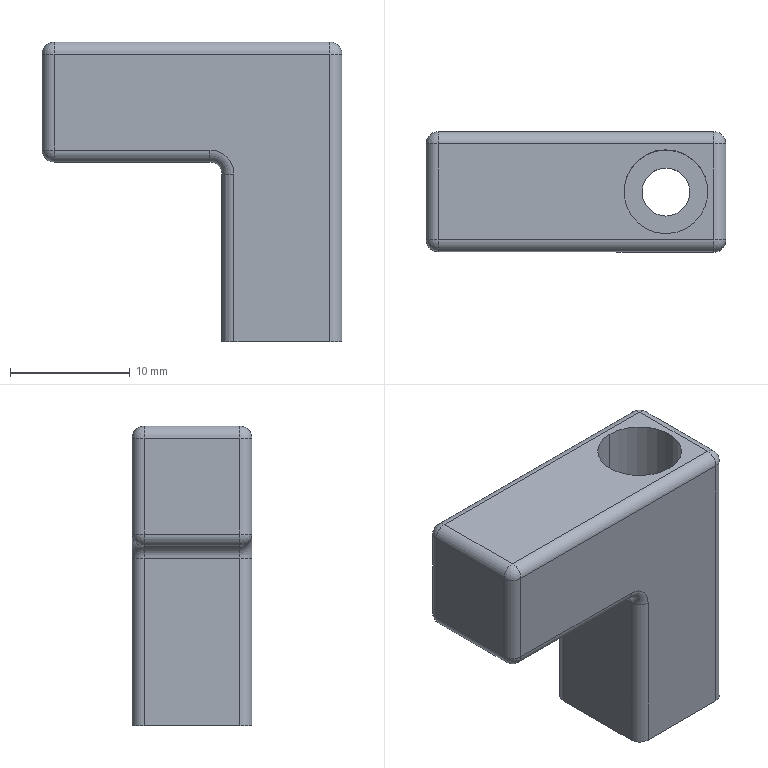Part | NX | 1 solid | 35 faces | box 25 x 10 x 25 mm | volume 3255 mm3 | cylinder 18 | plane 9 | sphere 6 | torus 2 | commonest cylinder face diameters 2 x14 4 x2 7 x2
STEP:
#1=CARTESIAN_POINT('',(12.5,-4.,-25.));
#2=VERTEX_POINT('',#1);
#3=CARTESIAN_POINT('',(12.5,4.,-25.));
#4=VERTEX_POINT('',#3);
#5=CARTESIAN_POINT('',(12.5,-4.,-25.));
#6=DIRECTION('',(0.,1.,0.));
#7=VECTOR('',#6,1000.);
#8=LINE('',#5,#7);
#9=EDGE_CURVE('',#2,#4,#8,.T.);
#10=ORIENTED_EDGE('',*,*,#9,.F.);
#11=CARTESIAN_POINT('',(11.5,-5.,-25.));
#12=VERTEX_POINT('',#11);
#13=CARTESIAN_POINT('',(11.5,-4.,-25.));
#14=DIRECTION('',(0.,0.,-1.));
#15=DIRECTION('',(1.,0.,0.));
#16=AXIS2_PLACEMENT_3D('',#13,#14,#15);
#17=CIRCLE('',#16,1.);
#18=EDGE_CURVE('',#2,#12,#17,.T.);
#19=ORIENTED_EDGE('',*,*,#18,.T.);
#20=CARTESIAN_POINT('',(3.5,-5.,-25.));
#21=VERTEX_POINT('',#20);
#22=CARTESIAN_POINT('',(3.5,-5.,-25.));
#23=DIRECTION('',(1.,0.,0.));
#24=VECTOR('',#23,1000.);
#25=LINE('',#22,#24);
#26=EDGE_CURVE('',#21,#12,#25,.T.);
#27=ORIENTED_EDGE('',*,*,#26,.F.);
#28=CARTESIAN_POINT('',(2.5,-4.,-25.));
#29=VERTEX_POINT('',#28);
#30=CARTESIAN_POINT('',(3.5,-4.,-25.));
#31=DIRECTION('',(0.,0.,-1.));
#32=DIRECTION('',(0.,-1.,0.));
#33=AXIS2_PLACEMENT_3D('',#30,#31,#32);
#34=CIRCLE('',#33,1.);
#35=EDGE_CURVE('',#21,#29,#34,.T.);
#36=ORIENTED_EDGE('',*,*,#35,.T.);
#37=CARTESIAN_POINT('',(2.5,4.,-25.));
#38=VERTEX_POINT('',#37);
#39=CARTESIAN_POINT('',(2.5,4.,-25.));
#40=DIRECTION('',(0.,-1.,0.));
#41=VECTOR('',#40,1000.);
#42=LINE('',#39,#41);
#43=EDGE_CURVE('',#38,#29,#42,.T.);
#44=ORIENTED_EDGE('',*,*,#43,.F.);
#45=CARTESIAN_POINT('',(3.5,5.,-25.));
#46=VERTEX_POINT('',#45);
#47=CARTESIAN_POINT('',(3.5,4.,-25.));
#48=DIRECTION('',(0.,0.,-1.));
#49=DIRECTION('',(-1.,0.,0.));
#50=AXIS2_PLACEMENT_3D('',#47,#48,#49);
#51=CIRCLE('',#50,1.);
#52=EDGE_CURVE('',#38,#46,#51,.T.);
#53=ORIENTED_EDGE('',*,*,#52,.T.);
#54=CARTESIAN_POINT('',(11.5,5.,-25.));
#55=VERTEX_POINT('',#54);
#56=CARTESIAN_POINT('',(11.5,5.,-25.));
#57=DIRECTION('',(-1.,0.,0.));
#58=VECTOR('',#57,1000.);
#59=LINE('',#56,#58);
#60=EDGE_CURVE('',#55,#46,#59,.T.);
#61=ORIENTED_EDGE('',*,*,#60,.F.);
#62=CARTESIAN_POINT('',(11.5,4.,-25.));
#63=DIRECTION('',(0.,0.,-1.));
#64=DIRECTION('',(0.,1.,0.));
#65=AXIS2_PLACEMENT_3D('',#62,#63,#64);
#66=CIRCLE('',#65,1.);
#67=EDGE_CURVE('',#55,#4,#66,.T.);
#68=ORIENTED_EDGE('',*,*,#67,.T.);
#69=EDGE_LOOP('',(#10,#19,#27,#36,#44,#53,#61,#68));
#70=FACE_BOUND('',#69,.T.);
#71=CARTESIAN_POINT('',(7.5,-2.,-25.));
#72=VERTEX_POINT('',#71);
#73=CARTESIAN_POINT('',(7.5,2.,-25.));
#74=VERTEX_POINT('',#73);
#75=CARTESIAN_POINT('',(7.5,0.,-25.));
#76=DIRECTION('',(0.,0.,1.));
#77=DIRECTION('',(0.,-1.,0.));
#78=AXIS2_PLACEMENT_3D('',#75,#76,#77);
#79=CIRCLE('',#78,2.);
#80=EDGE_CURVE('',#72,#74,#79,.T.);
#81=ORIENTED_EDGE('',*,*,#80,.T.);
#82=CARTESIAN_POINT('',(7.5,0.,-25.));
#83=DIRECTION('',(0.,0.,1.));
#84=DIRECTION('',(0.,1.,0.));
#85=AXIS2_PLACEMENT_3D('',#82,#83,#84);
#86=CIRCLE('',#85,2.);
#87=EDGE_CURVE('',#74,#72,#86,.T.);
#88=ORIENTED_EDGE('',*,*,#87,.T.);
#89=EDGE_LOOP('',(#81,#88));
#90=FACE_BOUND('',#89,.T.);
#91=CARTESIAN_POINT('',(2.5,-26.5,-25.));
#92=DIRECTION('',(0.,0.,1.));
#93=DIRECTION('',(0.,-1.,0.));
#94=AXIS2_PLACEMENT_3D('',#91,#92,#93);
#95=PLANE('',#94);
#96=ADVANCED_FACE('',(#70,#90),#95,.F.);
#97=CARTESIAN_POINT('',(12.5,4.,-1.));
#98=VERTEX_POINT('',#97);
#99=CARTESIAN_POINT('',(12.5,4.,-25.));
#100=DIRECTION('',(0.,0.,1.));
#101=VECTOR('',#100,1000.);
#102=LINE('',#99,#101);
#103=EDGE_CURVE('',#4,#98,#102,.T.);
#104=ORIENTED_EDGE('',*,*,#103,.F.);
#105=ORIENTED_EDGE('',*,*,#67,.F.);
#106=CARTESIAN_POINT('',(11.5,5.,-1.));
#107=VERTEX_POINT('',#106);
#108=CARTESIAN_POINT('',(11.5,5.,-25.));
#109=DIRECTION('',(0.,0.,1.));
#110=VECTOR('',#109,1000.);
#111=LINE('',#108,#110);
#112=EDGE_CURVE('',#55,#107,#111,.T.);
#113=ORIENTED_EDGE('',*,*,#112,.T.);
#114=CARTESIAN_POINT('',(11.5,4.,-1.));
#115=DIRECTION('',(0.,0.,1.));
#116=DIRECTION('',(1.,0.,0.));
#117=AXIS2_PLACEMENT_3D('',#114,#115,#116);
#118=CIRCLE('',#117,1.);
#119=EDGE_CURVE('',#98,#107,#118,.T.);
#120=ORIENTED_EDGE('',*,*,#119,.F.);
#121=EDGE_LOOP('',(#104,#105,#113,#120));
#122=FACE_BOUND('',#121,.T.);
#123=CARTESIAN_POINT('',(11.5,4.,-57.59));
#124=DIRECTION('',(0.,0.,1.));
#125=DIRECTION('',(-1.,0.,0.));
#126=AXIS2_PLACEMENT_3D('',#123,#124,#125);
#127=CYLINDRICAL_SURFACE('',#126,1.);
#128=ADVANCED_FACE('',(#122),#127,.T.);
#129=CARTESIAN_POINT('',(11.5,4.,0.));
#130=VERTEX_POINT('',#129);
#131=CARTESIAN_POINT('',(11.5,4.,-1.));
#132=DIRECTION('',(-1.,0.,0.));
#133=DIRECTION('',(0.,0.,1.));
#134=AXIS2_PLACEMENT_3D('',#131,#132,#133);
#135=CIRCLE('',#134,1.);
#136=EDGE_CURVE('',#130,#107,#135,.T.);
#137=ORIENTED_EDGE('',*,*,#136,.F.);
#138=CARTESIAN_POINT('',(11.5,4.,-1.));
#139=DIRECTION('',(0.,1.,0.));
#140=DIRECTION('',(0.,0.,1.));
#141=AXIS2_PLACEMENT_3D('',#138,#139,#140);
#142=CIRCLE('',#141,1.);
#143=EDGE_CURVE('',#130,#98,#142,.T.);
#144=ORIENTED_EDGE('',*,*,#143,.T.);
#145=ORIENTED_EDGE('',*,*,#119,.T.);
#146=EDGE_LOOP('',(#137,#144,#145));
#147=FACE_BOUND('',#146,.T.);
#148=CARTESIAN_POINT('',(11.5,4.,-1.));
#149=DIRECTION('',(0.7071,-0.7071,0.));
#150=DIRECTION('',(-0.7071,-0.7071,0.));
#151=AXIS2_PLACEMENT_3D('',#148,#149,#150);
#152=SPHERICAL_SURFACE('',#151,1.);
#153=ADVANCED_FACE('',(#147),#152,.T.);
#154=CARTESIAN_POINT('',(11.5,-4.,0.));
#155=VERTEX_POINT('',#154);
#156=CARTESIAN_POINT('',(12.5,-4.,-1.));
#157=VERTEX_POINT('',#156);
#158=CARTESIAN_POINT('',(11.5,-4.,-1.));
#159=DIRECTION('',(0.,1.,0.));
#160=DIRECTION('',(0.,0.,1.));
#161=AXIS2_PLACEMENT_3D('',#158,#159,#160);
#162=CIRCLE('',#161,1.);
#163=EDGE_CURVE('',#155,#157,#162,.T.);
#164=ORIENTED_EDGE('',*,*,#163,.T.);
#165=CARTESIAN_POINT('',(12.5,-4.,-1.));
#166=DIRECTION('',(0.,1.,0.));
#167=VECTOR('',#166,1000.);
#168=LINE('',#165,#167);
#169=EDGE_CURVE('',#157,#98,#168,.T.);
#170=ORIENTED_EDGE('',*,*,#169,.T.);
#171=ORIENTED_EDGE('',*,*,#143,.F.);
#172=CARTESIAN_POINT('',(11.5,-4.,0.));
#173=DIRECTION('',(0.,1.,0.));
#174=VECTOR('',#173,1000.);
#175=LINE('',#172,#174);
#176=EDGE_CURVE('',#155,#130,#175,.T.);
#177=ORIENTED_EDGE('',*,*,#176,.F.);
#178=EDGE_LOOP('',(#164,#170,#171,#177));
#179=FACE_BOUND('',#178,.T.);
#180=CARTESIAN_POINT('',(11.5,-4.056,-1.));
#181=DIRECTION('',(0.,1.,0.));
#182=DIRECTION('',(0.,0.,-1.));
#183=AXIS2_PLACEMENT_3D('',#180,#181,#182);
#184=CYLINDRICAL_SURFACE('',#183,1.);
#185=ADVANCED_FACE('',(#179),#184,.T.);
#186=CARTESIAN_POINT('',(-11.5,-4.,0.));
#187=VERTEX_POINT('',#186);
#188=CARTESIAN_POINT('',(-11.5,-4.,0.));
#189=DIRECTION('',(1.,0.,0.));
#190=VECTOR('',#189,1000.);
#191=LINE('',#188,#190);
#192=EDGE_CURVE('',#187,#155,#191,.T.);
#193=ORIENTED_EDGE('',*,*,#192,.T.);
#194=ORIENTED_EDGE('',*,*,#176,.T.);
#195=CARTESIAN_POINT('',(-11.5,4.,0.));
#196=VERTEX_POINT('',#195);
#197=CARTESIAN_POINT('',(11.5,4.,0.));
#198=DIRECTION('',(-1.,0.,0.));
#199=VECTOR('',#198,1000.);
#200=LINE('',#197,#199);
#201=EDGE_CURVE('',#130,#196,#200,.T.);
#202=ORIENTED_EDGE('',*,*,#201,.T.);
#203=CARTESIAN_POINT('',(-11.5,4.,0.));
#204=DIRECTION('',(0.,-1.,0.));
#205=VECTOR('',#204,1000.);
#206=LINE('',#203,#205);
#207=EDGE_CURVE('',#196,#187,#206,.T.);
#208=ORIENTED_EDGE('',*,*,#207,.T.);
#209=EDGE_LOOP('',(#193,#194,#202,#208));
#210=FACE_BOUND('',#209,.T.);
#211=CARTESIAN_POINT('',(7.5,-3.5,0.));
#212=VERTEX_POINT('',#211);
#213=CARTESIAN_POINT('',(7.5,3.5,0.));
#214=VERTEX_POINT('',#213);
#215=CARTESIAN_POINT('',(7.5,0.,0.));
#216=DIRECTION('',(0.,0.,1.));
#217=DIRECTION('',(0.,-1.,0.));
#218=AXIS2_PLACEMENT_3D('',#215,#216,#217);
#219=CIRCLE('',#218,3.5);
#220=EDGE_CURVE('',#212,#214,#219,.T.);
#221=ORIENTED_EDGE('',*,*,#220,.F.);
#222=CARTESIAN_POINT('',(7.5,0.,0.));
#223=DIRECTION('',(0.,0.,1.));
#224=DIRECTION('',(0.,1.,0.));
#225=AXIS2_PLACEMENT_3D('',#222,#223,#224);
#226=CIRCLE('',#225,3.5);
#227=EDGE_CURVE('',#214,#212,#226,.T.);
#228=ORIENTED_EDGE('',*,*,#227,.F.);
#229=EDGE_LOOP('',(#221,#228));
#230=FACE_BOUND('',#229,.T.);
#231=CARTESIAN_POINT('',(4.5,-26.5,0.));
#232=DIRECTION('',(0.,0.,1.));
#233=DIRECTION('',(0.,-1.,0.));
#234=AXIS2_PLACEMENT_3D('',#231,#232,#233);
#235=PLANE('',#234);
#236=ADVANCED_FACE('',(#210,#230),#235,.T.);
#237=CARTESIAN_POINT('',(7.5,-3.5,-15.));
#238=VERTEX_POINT('',#237);
#239=CARTESIAN_POINT('',(7.5,-3.5,0.));
#240=DIRECTION('',(0.,0.,-1.));
#241=VECTOR('',#240,1000.);
#242=LINE('',#239,#241);
#243=EDGE_CURVE('',#212,#238,#242,.T.);
#244=ORIENTED_EDGE('',*,*,#243,.T.);
#245=CARTESIAN_POINT('',(7.5,3.5,-15.));
#246=VERTEX_POINT('',#245);
#247=CARTESIAN_POINT('',(7.5,0.,-15.));
#248=DIRECTION('',(0.,0.,1.));
#249=DIRECTION('',(0.,1.,0.));
#250=AXIS2_PLACEMENT_3D('',#247,#248,#249);
#251=CIRCLE('',#250,3.5);
#252=EDGE_CURVE('',#246,#238,#251,.T.);
#253=ORIENTED_EDGE('',*,*,#252,.F.);
#254=CARTESIAN_POINT('',(7.5,3.5,0.));
#255=DIRECTION('',(0.,0.,-1.));
#256=VECTOR('',#255,1000.);
#257=LINE('',#254,#256);
#258=EDGE_CURVE('',#214,#246,#257,.T.);
#259=ORIENTED_EDGE('',*,*,#258,.F.);
#260=ORIENTED_EDGE('',*,*,#227,.T.);
#261=EDGE_LOOP('',(#244,#253,#259,#260));
#262=FACE_BOUND('',#261,.T.);
#263=CARTESIAN_POINT('',(7.5,0.,0.));
#264=DIRECTION('',(0.,0.,1.));
#265=DIRECTION('',(0.,-1.,0.));
#266=AXIS2_PLACEMENT_3D('',#263,#264,#265);
#267=CYLINDRICAL_SURFACE('',#266,3.5);
#268=ADVANCED_FACE('',(#262),#267,.F.);
#269=ORIENTED_EDGE('',*,*,#258,.T.);
#270=CARTESIAN_POINT('',(7.5,0.,-15.));
#271=DIRECTION('',(0.,0.,1.));
#272=DIRECTION('',(0.,-1.,0.));
#273=AXIS2_PLACEMENT_3D('',#270,#271,#272);
#274=CIRCLE('',#273,3.5);
#275=EDGE_CURVE('',#238,#246,#274,.T.);
#276=ORIENTED_EDGE('',*,*,#275,.F.);
#277=ORIENTED_EDGE('',*,*,#243,.F.);
#278=ORIENTED_EDGE('',*,*,#220,.T.);
#279=EDGE_LOOP('',(#269,#276,#277,#278));
#280=FACE_BOUND('',#279,.T.);
#281=CARTESIAN_POINT('',(7.5,0.,0.));
#282=DIRECTION('',(0.,0.,1.));
#283=DIRECTION('',(0.,-1.,0.));
#284=AXIS2_PLACEMENT_3D('',#281,#282,#283);
#285=CYLINDRICAL_SURFACE('',#284,3.5);
#286=ADVANCED_FACE('',(#280),#285,.F.);
#287=ORIENTED_EDGE('',*,*,#275,.T.);
#288=ORIENTED_EDGE('',*,*,#252,.T.);
#289=EDGE_LOOP('',(#287,#288));
#290=FACE_BOUND('',#289,.T.);
#291=CARTESIAN_POINT('',(7.5,-2.,-15.));
#292=VERTEX_POINT('',#291);
#293=CARTESIAN_POINT('',(7.5,2.,-15.));
#294=VERTEX_POINT('',#293);
#295=CARTESIAN_POINT('',(7.5,0.,-15.));
#296=DIRECTION('',(0.,0.,1.));
#297=DIRECTION('',(0.,-1.,0.));
#298=AXIS2_PLACEMENT_3D('',#295,#296,#297);
#299=CIRCLE('',#298,2.);
#300=EDGE_CURVE('',#292,#294,#299,.T.);
#301=ORIENTED_EDGE('',*,*,#300,.F.);
#302=CARTESIAN_POINT('',(7.5,0.,-15.));
#303=DIRECTION('',(0.,0.,1.));
#304=DIRECTION('',(0.,1.,0.));
#305=AXIS2_PLACEMENT_3D('',#302,#303,#304);
#306=CIRCLE('',#305,2.);
#307=EDGE_CURVE('',#294,#292,#306,.T.);
#308=ORIENTED_EDGE('',*,*,#307,.F.);
#309=EDGE_LOOP('',(#301,#308));
#310=FACE_BOUND('',#309,.T.);
#311=CARTESIAN_POINT('',(4.5,-26.5,-15.));
#312=DIRECTION('',(0.,0.,1.));
#313=DIRECTION('',(0.,-1.,0.));
#314=AXIS2_PLACEMENT_3D('',#311,#312,#313);
#315=PLANE('',#314);
#316=ADVANCED_FACE('',(#290,#310),#315,.T.);
#317=CARTESIAN_POINT('',(7.5,-2.,-15.));
#318=DIRECTION('',(0.,0.,-1.));
#319=VECTOR('',#318,1000.);
#320=LINE('',#317,#319);
#321=EDGE_CURVE('',#292,#72,#320,.T.);
#322=ORIENTED_EDGE('',*,*,#321,.T.);
#323=ORIENTED_EDGE('',*,*,#87,.F.);
#324=CARTESIAN_POINT('',(7.5,2.,-15.));
#325=DIRECTION('',(0.,0.,-1.));
#326=VECTOR('',#325,1000.);
#327=LINE('',#324,#326);
#328=EDGE_CURVE('',#294,#74,#327,.T.);
#329=ORIENTED_EDGE('',*,*,#328,.F.);
#330=ORIENTED_EDGE('',*,*,#307,.T.);
#331=EDGE_LOOP('',(#322,#323,#329,#330));
#332=FACE_BOUND('',#331,.T.);
#333=CARTESIAN_POINT('',(7.5,0.,0.));
#334=DIRECTION('',(0.,0.,1.));
#335=DIRECTION('',(0.,-1.,0.));
#336=AXIS2_PLACEMENT_3D('',#333,#334,#335);
#337=CYLINDRICAL_SURFACE('',#336,2.);
#338=ADVANCED_FACE('',(#332),#337,.F.);
#339=ORIENTED_EDGE('',*,*,#328,.T.);
#340=ORIENTED_EDGE('',*,*,#80,.F.);
#341=ORIENTED_EDGE('',*,*,#321,.F.);
#342=ORIENTED_EDGE('',*,*,#300,.T.);
#343=EDGE_LOOP('',(#339,#340,#341,#342));
#344=FACE_BOUND('',#343,.T.);
#345=CARTESIAN_POINT('',(7.5,0.,0.));
#346=DIRECTION('',(0.,0.,1.));
#347=DIRECTION('',(0.,-1.,0.));
#348=AXIS2_PLACEMENT_3D('',#345,#346,#347);
#349=CYLINDRICAL_SURFACE('',#348,2.);
#350=ADVANCED_FACE('',(#344),#349,.F.);
#351=CARTESIAN_POINT('',(-12.5,4.,-1.));
#352=VERTEX_POINT('',#351);
#353=CARTESIAN_POINT('',(-11.5,4.,-1.));
#354=DIRECTION('',(0.,-1.,0.));
#355=DIRECTION('',(0.,0.,1.));
#356=AXIS2_PLACEMENT_3D('',#353,#354,#355);
#357=CIRCLE('',#356,1.);
#358=EDGE_CURVE('',#196,#352,#357,.T.);
#359=ORIENTED_EDGE('',*,*,#358,.T.);
#360=CARTESIAN_POINT('',(-12.5,-4.,-1.));
#361=VERTEX_POINT('',#360);
#362=CARTESIAN_POINT('',(-12.5,4.,-1.));
#363=DIRECTION('',(0.,-1.,0.));
#364=VECTOR('',#363,1000.);
#365=LINE('',#362,#364);
#366=EDGE_CURVE('',#352,#361,#365,.T.);
#367=ORIENTED_EDGE('',*,*,#366,.T.);
#368=CARTESIAN_POINT('',(-11.5,-4.,-1.));
#369=DIRECTION('',(0.,-1.,0.));
#370=DIRECTION('',(0.,0.,1.));
#371=AXIS2_PLACEMENT_3D('',#368,#369,#370);
#372=CIRCLE('',#371,1.);
#373=EDGE_CURVE('',#187,#361,#372,.T.);
#374=ORIENTED_EDGE('',*,*,#373,.F.);
#375=ORIENTED_EDGE('',*,*,#207,.F.);
#376=EDGE_LOOP('',(#359,#367,#374,#375));
#377=FACE_BOUND('',#376,.T.);
#378=CARTESIAN_POINT('',(-11.5,4.056,-1.));
#379=DIRECTION('',(0.,-1.,0.));
#380=DIRECTION('',(0.,0.,-1.));
#381=AXIS2_PLACEMENT_3D('',#378,#379,#380);
#382=CYLINDRICAL_SURFACE('',#381,1.);
#383=ADVANCED_FACE('',(#377),#382,.T.);
#384=CARTESIAN_POINT('',(-11.5,-5.,-1.));
#385=VERTEX_POINT('',#384);
#386=CARTESIAN_POINT('',(-11.5,-4.,-1.));
#387=DIRECTION('',(1.,0.,0.));
#388=DIRECTION('',(0.,0.,1.));
#389=AXIS2_PLACEMENT_3D('',#386,#387,#388);
#390=CIRCLE('',#389,1.);
#391=EDGE_CURVE('',#187,#385,#390,.T.);
#392=ORIENTED_EDGE('',*,*,#391,.F.);
#393=ORIENTED_EDGE('',*,*,#373,.T.);
#394=CARTESIAN_POINT('',(-11.5,-4.,-1.));
#395=DIRECTION('',(0.,0.,1.));
#396=DIRECTION('',(-1.,0.,0.));
#397=AXIS2_PLACEMENT_3D('',#394,#395,#396);
#398=CIRCLE('',#397,1.);
#399=EDGE_CURVE('',#361,#385,#398,.T.);
#400=ORIENTED_EDGE('',*,*,#399,.T.);
#401=EDGE_LOOP('',(#392,#393,#400));
#402=FACE_BOUND('',#401,.T.);
#403=CARTESIAN_POINT('',(-11.5,-4.,-1.));
#404=DIRECTION('',(-0.7071,0.7071,0.));
#405=DIRECTION('',(0.7071,0.7071,0.));
#406=AXIS2_PLACEMENT_3D('',#403,#404,#405);
#407=SPHERICAL_SURFACE('',#406,1.);
#408=ADVANCED_FACE('',(#402),#407,.T.);
#409=CARTESIAN_POINT('',(-12.5,-4.,-9.));
#410=VERTEX_POINT('',#409);
#411=CARTESIAN_POINT('',(-12.5,-4.,-1.));
#412=DIRECTION('',(0.,0.,-1.));
#413=VECTOR('',#412,1000.);
#414=LINE('',#411,#413);
#415=EDGE_CURVE('',#361,#410,#414,.T.);
#416=ORIENTED_EDGE('',*,*,#415,.T.);
#417=CARTESIAN_POINT('',(-11.5,-5.,-9.));
#418=VERTEX_POINT('',#417);
#419=CARTESIAN_POINT('',(-11.5,-4.,-9.));
#420=DIRECTION('',(0.,0.,-1.));
#421=DIRECTION('',(0.,-1.,0.));
#422=AXIS2_PLACEMENT_3D('',#419,#420,#421);
#423=CIRCLE('',#422,1.);
#424=EDGE_CURVE('',#418,#410,#423,.T.);
#425=ORIENTED_EDGE('',*,*,#424,.F.);
#426=CARTESIAN_POINT('',(-11.5,-5.,-1.));
#427=DIRECTION('',(0.,0.,-1.));
#428=VECTOR('',#427,1000.);
#429=LINE('',#426,#428);
#430=EDGE_CURVE('',#385,#418,#429,.T.);
#431=ORIENTED_EDGE('',*,*,#430,.F.);
#432=ORIENTED_EDGE('',*,*,#399,.F.);
#433=EDGE_LOOP('',(#416,#425,#431,#432));
#434=FACE_BOUND('',#433,.T.);
#435=CARTESIAN_POINT('',(-11.5,-4.,32.59));
#436=DIRECTION('',(0.,0.,-1.));
#437=DIRECTION('',(0.,1.,0.));
#438=AXIS2_PLACEMENT_3D('',#435,#436,#437);
#439=CYLINDRICAL_SURFACE('',#438,1.);
#440=ADVANCED_FACE('',(#434),#439,.T.);
#441=ORIENTED_EDGE('',*,*,#26,.T.);
#442=CARTESIAN_POINT('',(11.5,-5.,-1.));
#443=VERTEX_POINT('',#442);
#444=CARTESIAN_POINT('',(11.5,-5.,-1.));
#445=DIRECTION('',(0.,0.,-1.));
#446=VECTOR('',#445,1000.);
#447=LINE('',#444,#446);
#448=EDGE_CURVE('',#443,#12,#447,.T.);
#449=ORIENTED_EDGE('',*,*,#448,.F.);
#450=CARTESIAN_POINT('',(-11.5,-5.,-1.));
#451=DIRECTION('',(1.,0.,0.));
#452=VECTOR('',#451,1000.);
#453=LINE('',#450,#452);
#454=EDGE_CURVE('',#385,#443,#453,.T.);
#455=ORIENTED_EDGE('',*,*,#454,.F.);
#456=ORIENTED_EDGE('',*,*,#430,.T.);
#457=CARTESIAN_POINT('',(1.5,-5.,-9.));
#458=VERTEX_POINT('',#457);
#459=CARTESIAN_POINT('',(1.5,-5.,-9.));
#460=DIRECTION('',(-1.,0.,0.));
#461=VECTOR('',#460,1000.);
#462=LINE('',#459,#461);
#463=EDGE_CURVE('',#458,#418,#462,.T.);
#464=ORIENTED_EDGE('',*,*,#463,.F.);
#465=CARTESIAN_POINT('',(3.5,-5.,-11.));
#466=VERTEX_POINT('',#465);
#467=CARTESIAN_POINT('',(1.5,-5.,-11.));
#468=DIRECTION('',(0.,-1.,0.));
#469=DIRECTION('',(1.,0.,0.));
#470=AXIS2_PLACEMENT_3D('',#467,#468,#469);
#471=CIRCLE('',#470,2.);
#472=EDGE_CURVE('',#466,#458,#471,.T.);
#473=ORIENTED_EDGE('',*,*,#472,.F.);
#474=CARTESIAN_POINT('',(3.5,-5.,-11.));
#475=DIRECTION('',(0.,0.,-1.));
#476=VECTOR('',#475,1000.);
#477=LINE('',#474,#476);
#478=EDGE_CURVE('',#466,#21,#477,.T.);
#479=ORIENTED_EDGE('',*,*,#478,.T.);
#480=EDGE_LOOP('',(#441,#449,#455,#456,#464,#473,#479));
#481=FACE_BOUND('',#480,.T.);
#482=CARTESIAN_POINT('',(2.5,-5.,-25.));
#483=DIRECTION('',(0.,-1.,0.));
#484=DIRECTION('',(-1.,0.,0.));
#485=AXIS2_PLACEMENT_3D('',#482,#483,#484);
#486=PLANE('',#485);
#487=ADVANCED_FACE('',(#481),#486,.T.);
#488=CARTESIAN_POINT('',(2.5,-4.,-11.));
#489=VERTEX_POINT('',#488);
#490=CARTESIAN_POINT('',(2.5,-4.,-11.));
#491=DIRECTION('',(0.,0.,-1.));
#492=VECTOR('',#491,1000.);
#493=LINE('',#490,#492);
#494=EDGE_CURVE('',#489,#29,#493,.T.);
#495=ORIENTED_EDGE('',*,*,#494,.T.);
#496=ORIENTED_EDGE('',*,*,#35,.F.);
#497=ORIENTED_EDGE('',*,*,#478,.F.);
#498=CARTESIAN_POINT('',(3.5,-4.,-11.));
#499=DIRECTION('',(0.,0.,1.));
#500=DIRECTION('',(-1.,0.,0.));
#501=AXIS2_PLACEMENT_3D('',#498,#499,#500);
#502=CIRCLE('',#501,1.);
#503=EDGE_CURVE('',#489,#466,#502,.T.);
#504=ORIENTED_EDGE('',*,*,#503,.F.);
#505=EDGE_LOOP('',(#495,#496,#497,#504));
#506=FACE_BOUND('',#505,.T.);
#507=CARTESIAN_POINT('',(3.5,-4.,32.59));
#508=DIRECTION('',(0.,0.,-1.));
#509=DIRECTION('',(0.,1.,0.));
#510=AXIS2_PLACEMENT_3D('',#507,#508,#509);
#511=CYLINDRICAL_SURFACE('',#510,1.);
#512=ADVANCED_FACE('',(#506),#511,.T.);
#513=CARTESIAN_POINT('',(1.5,-4.,-10.));
#514=VERTEX_POINT('',#513);
#515=CARTESIAN_POINT('',(1.5,-4.,-9.));
#516=DIRECTION('',(1.,0.,0.));
#517=DIRECTION('',(0.,-1.,0.));
#518=AXIS2_PLACEMENT_3D('',#515,#516,#517);
#519=CIRCLE('',#518,1.);
#520=EDGE_CURVE('',#458,#514,#519,.T.);
#521=ORIENTED_EDGE('',*,*,#520,.T.);
#522=CARTESIAN_POINT('',(1.5,-4.,-11.));
#523=DIRECTION('',(0.,1.,0.));
#524=DIRECTION('',(0.,0.,1.));
#525=AXIS2_PLACEMENT_3D('',#522,#523,#524);
#526=CIRCLE('',#525,1.);
#527=EDGE_CURVE('',#514,#489,#526,.T.);
#528=ORIENTED_EDGE('',*,*,#527,.T.);
#529=ORIENTED_EDGE('',*,*,#503,.T.);
#530=ORIENTED_EDGE('',*,*,#472,.T.);
#531=EDGE_LOOP('',(#521,#528,#529,#530));
#532=FACE_BOUND('',#531,.T.);
#533=CARTESIAN_POINT('',(1.5,-4.,-11.));
#534=DIRECTION('',(0.,-1.,0.));
#535=DIRECTION('',(-1.,0.,0.));
#536=AXIS2_PLACEMENT_3D('',#533,#534,#535);
#537=TOROIDAL_SURFACE('',#536,2.,1.);
#538=ADVANCED_FACE('',(#532),#537,.T.);
#539=CARTESIAN_POINT('',(2.5,4.,-11.));
#540=VERTEX_POINT('',#539);
#541=CARTESIAN_POINT('',(1.5,4.,-10.));
#542=VERTEX_POINT('',#541);
#543=CARTESIAN_POINT('',(1.5,4.,-11.));
#544=DIRECTION('',(0.,-1.,0.));
#545=DIRECTION('',(1.,0.,0.));
#546=AXIS2_PLACEMENT_3D('',#543,#544,#545);
#547=CIRCLE('',#546,1.);
#548=EDGE_CURVE('',#540,#542,#547,.T.);
#549=ORIENTED_EDGE('',*,*,#548,.F.);
#550=CARTESIAN_POINT('',(2.5,4.,-11.));
#551=DIRECTION('',(0.,-1.,0.));
#552=VECTOR('',#551,1000.);
#553=LINE('',#550,#552);
#554=EDGE_CURVE('',#540,#489,#553,.T.);
#555=ORIENTED_EDGE('',*,*,#554,.T.);
#556=ORIENTED_EDGE('',*,*,#527,.F.);
#557=CARTESIAN_POINT('',(1.5,4.,-10.));
#558=DIRECTION('',(0.,-1.,0.));
#559=VECTOR('',#558,1000.);
#560=LINE('',#557,#559);
#561=EDGE_CURVE('',#542,#514,#560,.T.);
#562=ORIENTED_EDGE('',*,*,#561,.F.);
#563=EDGE_LOOP('',(#549,#555,#556,#562));
#564=FACE_BOUND('',#563,.T.);
#565=CARTESIAN_POINT('',(1.5,4.059,-11.));
#566=DIRECTION('',(0.,-1.,0.));
#567=DIRECTION('',(-1.,0.,0.));
#568=AXIS2_PLACEMENT_3D('',#565,#566,#567);
#569=CYLINDRICAL_SURFACE('',#568,1.);
#570=ADVANCED_FACE('',(#564),#569,.F.);
#571=CARTESIAN_POINT('',(-11.5,-4.,-10.));
#572=VERTEX_POINT('',#571);
#573=CARTESIAN_POINT('',(1.5,-4.,-10.));
#574=DIRECTION('',(-1.,0.,0.));
#575=VECTOR('',#574,1000.);
#576=LINE('',#573,#575);
#577=EDGE_CURVE('',#514,#572,#576,.T.);
#578=ORIENTED_EDGE('',*,*,#577,.T.);
#579=CARTESIAN_POINT('',(-11.5,4.,-10.));
#580=VERTEX_POINT('',#579);
#581=CARTESIAN_POINT('',(-11.5,-4.,-10.));
#582=DIRECTION('',(0.,1.,0.));
#583=VECTOR('',#582,1000.);
#584=LINE('',#581,#583);
#585=EDGE_CURVE('',#572,#580,#584,.T.);
#586=ORIENTED_EDGE('',*,*,#585,.T.);
#587=CARTESIAN_POINT('',(-11.5,4.,-10.));
#588=DIRECTION('',(1.,0.,0.));
#589=VECTOR('',#588,1000.);
#590=LINE('',#587,#589);
#591=EDGE_CURVE('',#580,#542,#590,.T.);
#592=ORIENTED_EDGE('',*,*,#591,.T.);
#593=ORIENTED_EDGE('',*,*,#561,.T.);
#594=EDGE_LOOP('',(#578,#586,#592,#593));
#595=FACE_BOUND('',#594,.T.);
#596=CARTESIAN_POINT('',(4.5,-26.5,-10.));
#597=DIRECTION('',(0.,0.,1.));
#598=DIRECTION('',(0.,-1.,0.));
#599=AXIS2_PLACEMENT_3D('',#596,#597,#598);
#600=PLANE('',#599);
#601=ADVANCED_FACE('',(#595),#600,.F.);
#602=CARTESIAN_POINT('',(1.5,5.,-9.));
#603=VERTEX_POINT('',#602);
#604=CARTESIAN_POINT('',(1.5,4.,-9.));
#605=DIRECTION('',(1.,0.,0.));
#606=DIRECTION('',(0.,0.,-1.));
#607=AXIS2_PLACEMENT_3D('',#604,#605,#606);
#608=CIRCLE('',#607,1.);
#609=EDGE_CURVE('',#542,#603,#608,.T.);
#610=ORIENTED_EDGE('',*,*,#609,.F.);
#611=ORIENTED_EDGE('',*,*,#591,.F.);
#612=CARTESIAN_POINT('',(-11.5,5.,-9.));
#613=VERTEX_POINT('',#612);
#614=CARTESIAN_POINT('',(-11.5,4.,-9.));
#615=DIRECTION('',(1.,0.,0.));
#616=DIRECTION('',(0.,0.,-1.));
#617=AXIS2_PLACEMENT_3D('',#614,#615,#616);
#618=CIRCLE('',#617,1.);
#619=EDGE_CURVE('',#580,#613,#618,.T.);
#620=ORIENTED_EDGE('',*,*,#619,.T.);
#621=CARTESIAN_POINT('',(-11.5,5.,-9.));
#622=DIRECTION('',(1.,0.,0.));
#623=VECTOR('',#622,1000.);
#624=LINE('',#621,#623);
#625=EDGE_CURVE('',#613,#603,#624,.T.);
#626=ORIENTED_EDGE('',*,*,#625,.T.);
#627=EDGE_LOOP('',(#610,#611,#620,#626));
#628=FACE_BOUND('',#627,.T.);
#629=CARTESIAN_POINT('',(-11.58,4.,-9.));
#630=DIRECTION('',(1.,0.,0.));
#631=DIRECTION('',(0.,0.,1.));
#632=AXIS2_PLACEMENT_3D('',#629,#630,#631);
#633=CYLINDRICAL_SURFACE('',#632,1.);
#634=ADVANCED_FACE('',(#628),#633,.T.);
#635=ORIENTED_EDGE('',*,*,#625,.F.);
#636=CARTESIAN_POINT('',(-11.5,5.,-1.));
#637=VERTEX_POINT('',#636);
#638=CARTESIAN_POINT('',(-11.5,5.,-1.));
#639=DIRECTION('',(0.,0.,-1.));
#640=VECTOR('',#639,1000.);
#641=LINE('',#638,#640);
#642=EDGE_CURVE('',#637,#613,#641,.T.);
#643=ORIENTED_EDGE('',*,*,#642,.F.);
#644=CARTESIAN_POINT('',(11.5,5.,-1.));
#645=DIRECTION('',(-1.,0.,0.));
#646=VECTOR('',#645,1000.);
#647=LINE('',#644,#646);
#648=EDGE_CURVE('',#107,#637,#647,.T.);
#649=ORIENTED_EDGE('',*,*,#648,.F.);
#650=ORIENTED_EDGE('',*,*,#112,.F.);
#651=ORIENTED_EDGE('',*,*,#60,.T.);
#652=CARTESIAN_POINT('',(3.5,5.,-11.));
#653=VERTEX_POINT('',#652);
#654=CARTESIAN_POINT('',(3.5,5.,-11.));
#655=DIRECTION('',(0.,0.,-1.));
#656=VECTOR('',#655,1000.);
#657=LINE('',#654,#656);
#658=EDGE_CURVE('',#653,#46,#657,.T.);
#659=ORIENTED_EDGE('',*,*,#658,.F.);
#660=CARTESIAN_POINT('',(1.5,5.,-11.));
#661=DIRECTION('',(0.,1.,0.));
#662=DIRECTION('',(0.,0.,1.));
#663=AXIS2_PLACEMENT_3D('',#660,#661,#662);
#664=CIRCLE('',#663,2.);
#665=EDGE_CURVE('',#603,#653,#664,.T.);
#666=ORIENTED_EDGE('',*,*,#665,.F.);
#667=EDGE_LOOP('',(#635,#643,#649,#650,#651,#659,#666));
#668=FACE_BOUND('',#667,.T.);
#669=CARTESIAN_POINT('',(12.5,5.,-25.));
#670=DIRECTION('',(0.,1.,0.));
#671=DIRECTION('',(1.,0.,0.));
#672=AXIS2_PLACEMENT_3D('',#669,#670,#671);
#673=PLANE('',#672);
#674=ADVANCED_FACE('',(#668),#673,.T.);
#675=ORIENTED_EDGE('',*,*,#548,.T.);
#676=ORIENTED_EDGE('',*,*,#609,.T.);
#677=ORIENTED_EDGE('',*,*,#665,.T.);
#678=CARTESIAN_POINT('',(3.5,4.,-11.));
#679=DIRECTION('',(0.,0.,-1.));
#680=DIRECTION('',(-1.,0.,0.));
#681=AXIS2_PLACEMENT_3D('',#678,#679,#680);
#682=CIRCLE('',#681,1.);
#683=EDGE_CURVE('',#540,#653,#682,.T.);
#684=ORIENTED_EDGE('',*,*,#683,.F.);
#685=EDGE_LOOP('',(#675,#676,#677,#684));
#686=FACE_BOUND('',#685,.T.);
#687=CARTESIAN_POINT('',(1.5,4.,-11.));
#688=DIRECTION('',(0.,-1.,0.));
#689=DIRECTION('',(0.,0.,-1.));
#690=AXIS2_PLACEMENT_3D('',#687,#688,#689);
#691=TOROIDAL_SURFACE('',#690,2.,1.);
#692=ADVANCED_FACE('',(#686),#691,.T.);
#693=ORIENTED_EDGE('',*,*,#658,.T.);
#694=ORIENTED_EDGE('',*,*,#52,.F.);
#695=CARTESIAN_POINT('',(2.5,4.,-11.));
#696=DIRECTION('',(0.,0.,-1.));
#697=VECTOR('',#696,1000.);
#698=LINE('',#695,#697);
#699=EDGE_CURVE('',#540,#38,#698,.T.);
#700=ORIENTED_EDGE('',*,*,#699,.F.);
#701=ORIENTED_EDGE('',*,*,#683,.T.);
#702=EDGE_LOOP('',(#693,#694,#700,#701));
#703=FACE_BOUND('',#702,.T.);
#704=CARTESIAN_POINT('',(3.5,4.,32.59));
#705=DIRECTION('',(0.,0.,-1.));
#706=DIRECTION('',(1.,0.,0.));
#707=AXIS2_PLACEMENT_3D('',#704,#705,#706);
#708=CYLINDRICAL_SURFACE('',#707,1.);
#709=ADVANCED_FACE('',(#703),#708,.T.);
#710=ORIENTED_EDGE('',*,*,#699,.T.);
#711=ORIENTED_EDGE('',*,*,#43,.T.);
#712=ORIENTED_EDGE('',*,*,#494,.F.);
#713=ORIENTED_EDGE('',*,*,#554,.F.);
#714=EDGE_LOOP('',(#710,#711,#712,#713));
#715=FACE_BOUND('',#714,.T.);
#716=CARTESIAN_POINT('',(2.5,5.,-25.));
#717=DIRECTION('',(-1.,0.,0.));
#718=DIRECTION('',(0.,1.,0.));
#719=AXIS2_PLACEMENT_3D('',#716,#717,#718);
#720=PLANE('',#719);
#721=ADVANCED_FACE('',(#715),#720,.T.);
#722=ORIENTED_EDGE('',*,*,#136,.T.);
#723=ORIENTED_EDGE('',*,*,#648,.T.);
#724=CARTESIAN_POINT('',(-11.5,4.,-1.));
#725=DIRECTION('',(-1.,0.,0.));
#726=DIRECTION('',(0.,0.,1.));
#727=AXIS2_PLACEMENT_3D('',#724,#725,#726);
#728=CIRCLE('',#727,1.);
#729=EDGE_CURVE('',#196,#637,#728,.T.);
#730=ORIENTED_EDGE('',*,*,#729,.F.);
#731=ORIENTED_EDGE('',*,*,#201,.F.);
#732=EDGE_LOOP('',(#722,#723,#730,#731));
#733=FACE_BOUND('',#732,.T.);
#734=CARTESIAN_POINT('',(11.556,4.,-1.));
#735=DIRECTION('',(-1.,0.,0.));
#736=DIRECTION('',(0.,0.,-1.));
#737=AXIS2_PLACEMENT_3D('',#734,#735,#736);
#738=CYLINDRICAL_SURFACE('',#737,1.);
#739=ADVANCED_FACE('',(#733),#738,.T.);
#740=ORIENTED_EDGE('',*,*,#358,.F.);
#741=ORIENTED_EDGE('',*,*,#729,.T.);
#742=CARTESIAN_POINT('',(-11.5,4.,-1.));
#743=DIRECTION('',(0.,0.,1.));
#744=DIRECTION('',(0.,1.,0.));
#745=AXIS2_PLACEMENT_3D('',#742,#743,#744);
#746=CIRCLE('',#745,1.);
#747=EDGE_CURVE('',#637,#352,#746,.T.);
#748=ORIENTED_EDGE('',*,*,#747,.T.);
#749=EDGE_LOOP('',(#740,#741,#748));
#750=FACE_BOUND('',#749,.T.);
#751=CARTESIAN_POINT('',(-11.5,4.,-1.));
#752=DIRECTION('',(0.7071,0.7071,0.));
#753=DIRECTION('',(0.7071,-0.7071,0.));
#754=AXIS2_PLACEMENT_3D('',#751,#752,#753);
#755=SPHERICAL_SURFACE('',#754,1.);
#756=ADVANCED_FACE('',(#750),#755,.T.);
#757=ORIENTED_EDGE('',*,*,#642,.T.);
#758=CARTESIAN_POINT('',(-12.5,4.,-9.));
#759=VERTEX_POINT('',#758);
#760=CARTESIAN_POINT('',(-11.5,4.,-9.));
#761=DIRECTION('',(0.,0.,-1.));
#762=DIRECTION('',(-1.,0.,0.));
#763=AXIS2_PLACEMENT_3D('',#760,#761,#762);
#764=CIRCLE('',#763,1.);
#765=EDGE_CURVE('',#759,#613,#764,.T.);
#766=ORIENTED_EDGE('',*,*,#765,.F.);
#767=CARTESIAN_POINT('',(-12.5,4.,-1.));
#768=DIRECTION('',(0.,0.,-1.));
#769=VECTOR('',#768,1000.);
#770=LINE('',#767,#769);
#771=EDGE_CURVE('',#352,#759,#770,.T.);
#772=ORIENTED_EDGE('',*,*,#771,.F.);
#773=ORIENTED_EDGE('',*,*,#747,.F.);
#774=EDGE_LOOP('',(#757,#766,#772,#773));
#775=FACE_BOUND('',#774,.T.);
#776=CARTESIAN_POINT('',(-11.5,4.,32.59));
#777=DIRECTION('',(0.,0.,-1.));
#778=DIRECTION('',(1.,0.,0.));
#779=AXIS2_PLACEMENT_3D('',#776,#777,#778);
#780=CYLINDRICAL_SURFACE('',#779,1.);
#781=ADVANCED_FACE('',(#775),#780,.T.);
#782=ORIENTED_EDGE('',*,*,#771,.T.);
#783=CARTESIAN_POINT('',(-12.5,-4.,-9.));
#784=DIRECTION('',(0.,1.,0.));
#785=VECTOR('',#784,1000.);
#786=LINE('',#783,#785);
#787=EDGE_CURVE('',#410,#759,#786,.T.);
#788=ORIENTED_EDGE('',*,*,#787,.F.);
#789=ORIENTED_EDGE('',*,*,#415,.F.);
#790=ORIENTED_EDGE('',*,*,#366,.F.);
#791=EDGE_LOOP('',(#782,#788,#789,#790));
#792=FACE_BOUND('',#791,.T.);
#793=CARTESIAN_POINT('',(-12.5,5.,-10.));
#794=DIRECTION('',(-1.,0.,0.));
#795=DIRECTION('',(0.,1.,0.));
#796=AXIS2_PLACEMENT_3D('',#793,#794,#795);
#797=PLANE('',#796);
#798=ADVANCED_FACE('',(#792),#797,.T.);
#799=CARTESIAN_POINT('',(-11.5,-4.,-9.));
#800=DIRECTION('',(0.,1.,0.));
#801=DIRECTION('',(0.,0.,-1.));
#802=AXIS2_PLACEMENT_3D('',#799,#800,#801);
#803=CIRCLE('',#802,1.);
#804=EDGE_CURVE('',#572,#410,#803,.T.);
#805=ORIENTED_EDGE('',*,*,#804,.T.);
#806=ORIENTED_EDGE('',*,*,#787,.T.);
#807=CARTESIAN_POINT('',(-11.5,4.,-9.));
#808=DIRECTION('',(0.,1.,0.));
#809=DIRECTION('',(0.,0.,-1.));
#810=AXIS2_PLACEMENT_3D('',#807,#808,#809);
#811=CIRCLE('',#810,1.);
#812=EDGE_CURVE('',#580,#759,#811,.T.);
#813=ORIENTED_EDGE('',*,*,#812,.F.);
#814=ORIENTED_EDGE('',*,*,#585,.F.);
#815=EDGE_LOOP('',(#805,#806,#813,#814));
#816=FACE_BOUND('',#815,.T.);
#817=CARTESIAN_POINT('',(-11.5,-4.08,-9.));
#818=DIRECTION('',(0.,1.,0.));
#819=DIRECTION('',(0.,0.,1.));
#820=AXIS2_PLACEMENT_3D('',#817,#818,#819);
#821=CYLINDRICAL_SURFACE('',#820,1.);
#822=ADVANCED_FACE('',(#816),#821,.T.);
#823=ORIENTED_EDGE('',*,*,#619,.F.);
#824=ORIENTED_EDGE('',*,*,#812,.T.);
#825=ORIENTED_EDGE('',*,*,#765,.T.);
#826=EDGE_LOOP('',(#823,#824,#825));
#827=FACE_BOUND('',#826,.T.);
#828=CARTESIAN_POINT('',(-11.5,4.,-9.));
#829=DIRECTION('',(-0.7071,-0.7071,0.));
#830=DIRECTION('',(0.7071,-0.7071,0.));
#831=AXIS2_PLACEMENT_3D('',#828,#829,#830);
#832=SPHERICAL_SURFACE('',#831,1.);
#833=ADVANCED_FACE('',(#827),#832,.T.);
#834=ORIENTED_EDGE('',*,*,#804,.F.);
#835=CARTESIAN_POINT('',(-11.5,-4.,-9.));
#836=DIRECTION('',(-1.,0.,0.));
#837=DIRECTION('',(0.,0.,-1.));
#838=AXIS2_PLACEMENT_3D('',#835,#836,#837);
#839=CIRCLE('',#838,1.);
#840=EDGE_CURVE('',#572,#418,#839,.T.);
#841=ORIENTED_EDGE('',*,*,#840,.T.);
#842=ORIENTED_EDGE('',*,*,#424,.T.);
#843=EDGE_LOOP('',(#834,#841,#842));
#844=FACE_BOUND('',#843,.T.);
#845=CARTESIAN_POINT('',(-11.5,-4.,-9.));
#846=DIRECTION('',(0.7071,-0.7071,0.));
#847=DIRECTION('',(0.7071,0.7071,0.));
#848=AXIS2_PLACEMENT_3D('',#845,#846,#847);
#849=SPHERICAL_SURFACE('',#848,1.);
#850=ADVANCED_FACE('',(#844),#849,.T.);
#851=ORIENTED_EDGE('',*,*,#520,.F.);
#852=ORIENTED_EDGE('',*,*,#463,.T.);
#853=ORIENTED_EDGE('',*,*,#840,.F.);
#854=ORIENTED_EDGE('',*,*,#577,.F.);
#855=EDGE_LOOP('',(#851,#852,#853,#854));
#856=FACE_BOUND('',#855,.T.);
#857=CARTESIAN_POINT('',(45.09,-4.,-9.));
#858=DIRECTION('',(-1.,0.,0.));
#859=DIRECTION('',(0.,0.,1.));
#860=AXIS2_PLACEMENT_3D('',#857,#858,#859);
#861=CYLINDRICAL_SURFACE('',#860,1.);
#862=ADVANCED_FACE('',(#856),#861,.T.);
#863=ORIENTED_EDGE('',*,*,#391,.T.);
#864=ORIENTED_EDGE('',*,*,#454,.T.);
#865=CARTESIAN_POINT('',(11.5,-4.,-1.));
#866=DIRECTION('',(1.,0.,0.));
#867=DIRECTION('',(0.,0.,1.));
#868=AXIS2_PLACEMENT_3D('',#865,#866,#867);
#869=CIRCLE('',#868,1.);
#870=EDGE_CURVE('',#155,#443,#869,.T.);
#871=ORIENTED_EDGE('',*,*,#870,.F.);
#872=ORIENTED_EDGE('',*,*,#192,.F.);
#873=EDGE_LOOP('',(#863,#864,#871,#872));
#874=FACE_BOUND('',#873,.T.);
#875=CARTESIAN_POINT('',(-11.556,-4.,-1.));
#876=DIRECTION('',(1.,0.,0.));
#877=DIRECTION('',(0.,0.,-1.));
#878=AXIS2_PLACEMENT_3D('',#875,#876,#877);
#879=CYLINDRICAL_SURFACE('',#878,1.);
#880=ADVANCED_FACE('',(#874),#879,.T.);
#881=ORIENTED_EDGE('',*,*,#163,.F.);
#882=ORIENTED_EDGE('',*,*,#870,.T.);
#883=CARTESIAN_POINT('',(11.5,-4.,-1.));
#884=DIRECTION('',(0.,0.,1.));
#885=DIRECTION('',(0.,-1.,0.));
#886=AXIS2_PLACEMENT_3D('',#883,#884,#885);
#887=CIRCLE('',#886,1.);
#888=EDGE_CURVE('',#443,#157,#887,.T.);
#889=ORIENTED_EDGE('',*,*,#888,.T.);
#890=EDGE_LOOP('',(#881,#882,#889));
#891=FACE_BOUND('',#890,.T.);
#892=CARTESIAN_POINT('',(11.5,-4.,-1.));
#893=DIRECTION('',(-0.7071,-0.7071,0.));
#894=DIRECTION('',(-0.7071,0.7071,0.));
#895=AXIS2_PLACEMENT_3D('',#892,#893,#894);
#896=SPHERICAL_SURFACE('',#895,1.);
#897=ADVANCED_FACE('',(#891),#896,.T.);
#898=ORIENTED_EDGE('',*,*,#448,.T.);
#899=ORIENTED_EDGE('',*,*,#18,.F.);
#900=CARTESIAN_POINT('',(12.5,-4.,-1.));
#901=DIRECTION('',(0.,0.,-1.));
#902=VECTOR('',#901,1000.);
#903=LINE('',#900,#902);
#904=EDGE_CURVE('',#157,#2,#903,.T.);
#905=ORIENTED_EDGE('',*,*,#904,.F.);
#906=ORIENTED_EDGE('',*,*,#888,.F.);
#907=EDGE_LOOP('',(#898,#899,#905,#906));
#908=FACE_BOUND('',#907,.T.);
#909=CARTESIAN_POINT('',(11.5,-4.,32.59));
#910=DIRECTION('',(0.,0.,-1.));
#911=DIRECTION('',(-1.,0.,0.));
#912=AXIS2_PLACEMENT_3D('',#909,#910,#911);
#913=CYLINDRICAL_SURFACE('',#912,1.);
#914=ADVANCED_FACE('',(#908),#913,.T.);
#915=ORIENTED_EDGE('',*,*,#904,.T.);
#916=ORIENTED_EDGE('',*,*,#9,.T.);
#917=ORIENTED_EDGE('',*,*,#103,.T.);
#918=ORIENTED_EDGE('',*,*,#169,.F.);
#919=EDGE_LOOP('',(#915,#916,#917,#918));
#920=FACE_BOUND('',#919,.T.);
#921=CARTESIAN_POINT('',(12.5,-5.,-25.));
#922=DIRECTION('',(1.,0.,0.));
#923=DIRECTION('',(0.,-1.,0.));
#924=AXIS2_PLACEMENT_3D('',#921,#922,#923);
#925=PLANE('',#924);
#926=ADVANCED_FACE('',(#920),#925,.T.);
#927=CLOSED_SHELL('',(#96,#128,#153,#185,#236,#268,#286,#316,#338,#350,#383,#408,#440,#487,#512,#538,#570,#601,#634,#674,#692,#709,#721,#739,#756,#781,#798,#822,#833,#850,#862,#880,#897,#914,#926));
#928=MANIFOLD_SOLID_BREP('',#927);
#929=(LENGTH_UNIT()NAMED_UNIT(*)SI_UNIT(.MILLI.,.METRE.));
#930=UNCERTAINTY_MEASURE_WITH_UNIT(LENGTH_MEASURE(0.00001),#929,'','');
#931=(NAMED_UNIT(*)PLANE_ANGLE_UNIT()SI_UNIT($,.RADIAN.));
#932=(NAMED_UNIT(*)SI_UNIT($,.STERADIAN.)SOLID_ANGLE_UNIT());
#933=(GEOMETRIC_REPRESENTATION_CONTEXT(3)GLOBAL_UNCERTAINTY_ASSIGNED_CONTEXT((#930))GLOBAL_UNIT_ASSIGNED_CONTEXT((#929,#931,#932))REPRESENTATION_CONTEXT('',''));
#934=ADVANCED_BREP_SHAPE_REPRESENTATION('',(#928),#933);